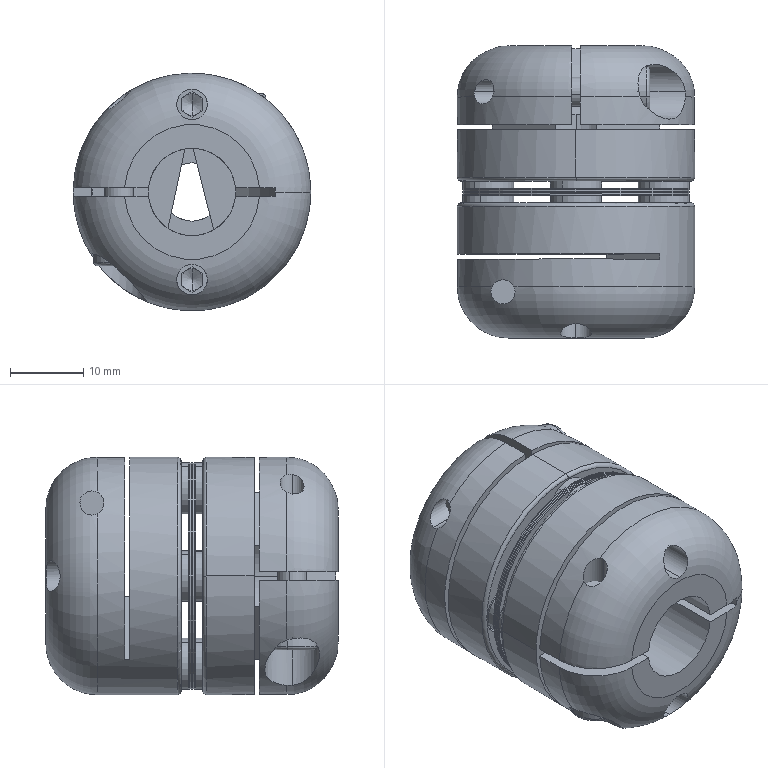Part | SolidWorks | features BaseBody 23 | 23 solids | 387 faces | box 32.5 x 40 x 32.5 mm | volume 24280 mm3 | cylinder 182 | plane 154 | cone 32 | torus 19 | commonest cylinder face diameters 4.1 x40 4.2 x36 7 x28 3.3 x12 4 x12 7.5 x12